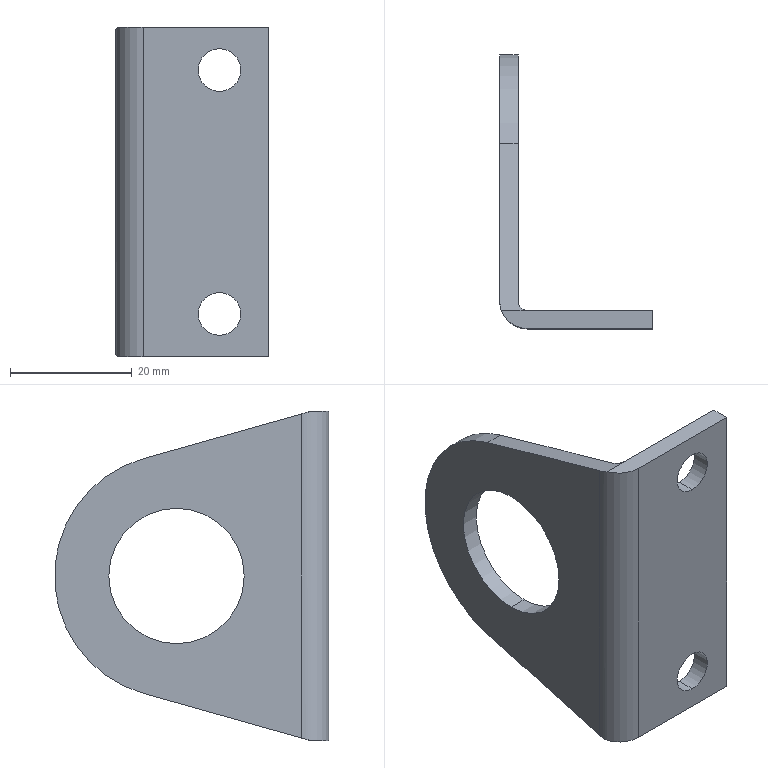Part | SolidWorks | features BaseBody 1 | 1 solid | 18 faces | box 25 x 45 x 54 mm | volume 7496 mm3 | cylinder 9 | plane 9 | commonest cylinder face diameters 7 x4 22.2 x2 3 x1 9 x1 40 x1
STEP:
#1=CARTESIAN_POINT('',(17.,-22.,16.5));
#2=VERTEX_POINT('',#1);
#3=CARTESIAN_POINT('',(17.,-22.,23.5));
#4=VERTEX_POINT('',#3);
#5=CARTESIAN_POINT('',(17.,-22.,20.));
#6=DIRECTION('',(0.,1.,0.));
#7=DIRECTION('',(1.,0.,0.));
#8=AXIS2_PLACEMENT_3D('',#5,#6,#7);
#9=CIRCLE('',#8,3.5);
#10=EDGE_CURVE('',#2,#4,#9,.T.);
#11=ORIENTED_EDGE('',*,*,#10,.T.);
#12=CARTESIAN_POINT('',(17.,-25.,23.5));
#13=VERTEX_POINT('',#12);
#14=CARTESIAN_POINT('',(17.,-22.,23.5));
#15=DIRECTION('',(0.,-1.,0.));
#16=VECTOR('',#15,1000.);
#17=LINE('',#14,#16);
#18=EDGE_CURVE('',#4,#13,#17,.T.);
#19=ORIENTED_EDGE('',*,*,#18,.T.);
#20=CARTESIAN_POINT('',(17.,-25.,16.5));
#21=VERTEX_POINT('',#20);
#22=CARTESIAN_POINT('',(17.,-25.,20.));
#23=DIRECTION('',(0.,-1.,0.));
#24=DIRECTION('',(0.,0.,1.));
#25=AXIS2_PLACEMENT_3D('',#22,#23,#24);
#26=CIRCLE('',#25,3.5);
#27=EDGE_CURVE('',#13,#21,#26,.T.);
#28=ORIENTED_EDGE('',*,*,#27,.T.);
#29=CARTESIAN_POINT('',(17.,-22.,16.5));
#30=DIRECTION('',(0.,-1.,0.));
#31=VECTOR('',#30,1000.);
#32=LINE('',#29,#31);
#33=EDGE_CURVE('',#2,#21,#32,.T.);
#34=ORIENTED_EDGE('',*,*,#33,.F.);
#35=EDGE_LOOP('',(#11,#19,#28,#34));
#36=FACE_OUTER_BOUND('',#35,.T.);
#37=CARTESIAN_POINT('',(17.,-22.,20.));
#38=DIRECTION('',(0.,-1.,0.));
#39=DIRECTION('',(0.,0.,-1.));
#40=AXIS2_PLACEMENT_3D('',#37,#38,#39);
#41=CYLINDRICAL_SURFACE('',#40,3.5);
#42=ADVANCED_FACE('',(#36),#41,.F.);
#43=CARTESIAN_POINT('',(17.,-22.,-23.5));
#44=VERTEX_POINT('',#43);
#45=CARTESIAN_POINT('',(17.,-22.,-16.5));
#46=VERTEX_POINT('',#45);
#47=CARTESIAN_POINT('',(17.,-22.,-20.));
#48=DIRECTION('',(0.,1.,0.));
#49=DIRECTION('',(1.,0.,0.));
#50=AXIS2_PLACEMENT_3D('',#47,#48,#49);
#51=CIRCLE('',#50,3.5);
#52=EDGE_CURVE('',#44,#46,#51,.T.);
#53=ORIENTED_EDGE('',*,*,#52,.T.);
#54=CARTESIAN_POINT('',(17.,-25.,-16.5));
#55=VERTEX_POINT('',#54);
#56=CARTESIAN_POINT('',(17.,-22.,-16.5));
#57=DIRECTION('',(0.,-1.,0.));
#58=VECTOR('',#57,1000.);
#59=LINE('',#56,#58);
#60=EDGE_CURVE('',#46,#55,#59,.T.);
#61=ORIENTED_EDGE('',*,*,#60,.T.);
#62=CARTESIAN_POINT('',(17.,-25.,-23.5));
#63=VERTEX_POINT('',#62);
#64=CARTESIAN_POINT('',(17.,-25.,-20.));
#65=DIRECTION('',(0.,-1.,0.));
#66=DIRECTION('',(0.,0.,1.));
#67=AXIS2_PLACEMENT_3D('',#64,#65,#66);
#68=CIRCLE('',#67,3.5);
#69=EDGE_CURVE('',#55,#63,#68,.T.);
#70=ORIENTED_EDGE('',*,*,#69,.T.);
#71=CARTESIAN_POINT('',(17.,-22.,-23.5));
#72=DIRECTION('',(0.,-1.,0.));
#73=VECTOR('',#72,1000.);
#74=LINE('',#71,#73);
#75=EDGE_CURVE('',#44,#63,#74,.T.);
#76=ORIENTED_EDGE('',*,*,#75,.F.);
#77=EDGE_LOOP('',(#53,#61,#70,#76));
#78=FACE_OUTER_BOUND('',#77,.T.);
#79=CARTESIAN_POINT('',(17.,-22.,-20.));
#80=DIRECTION('',(0.,-1.,0.));
#81=DIRECTION('',(0.,0.,-1.));
#82=AXIS2_PLACEMENT_3D('',#79,#80,#81);
#83=CYLINDRICAL_SURFACE('',#82,3.5);
#84=ADVANCED_FACE('',(#78),#83,.F.);
#85=CARTESIAN_POINT('',(3.,0.,11.1));
#86=VERTEX_POINT('',#85);
#87=CARTESIAN_POINT('',(3.,0.,-11.1));
#88=VERTEX_POINT('',#87);
#89=CARTESIAN_POINT('',(3.,0.,0.));
#90=DIRECTION('',(1.,0.,0.));
#91=DIRECTION('',(0.,0.,-1.));
#92=AXIS2_PLACEMENT_3D('',#89,#90,#91);
#93=CIRCLE('',#92,11.1);
#94=EDGE_CURVE('',#86,#88,#93,.T.);
#95=ORIENTED_EDGE('',*,*,#94,.T.);
#96=CARTESIAN_POINT('',(0.,0.,-11.1));
#97=VERTEX_POINT('',#96);
#98=CARTESIAN_POINT('',(3.,0.,-11.1));
#99=DIRECTION('',(-1.,0.,0.));
#100=VECTOR('',#99,1000.);
#101=LINE('',#98,#100);
#102=EDGE_CURVE('',#88,#97,#101,.T.);
#103=ORIENTED_EDGE('',*,*,#102,.T.);
#104=CARTESIAN_POINT('',(0.,0.,11.1));
#105=VERTEX_POINT('',#104);
#106=CARTESIAN_POINT('',(0.,0.,0.));
#107=DIRECTION('',(-1.,0.,0.));
#108=DIRECTION('',(0.,0.,-1.));
#109=AXIS2_PLACEMENT_3D('',#106,#107,#108);
#110=CIRCLE('',#109,11.1);
#111=EDGE_CURVE('',#97,#105,#110,.T.);
#112=ORIENTED_EDGE('',*,*,#111,.T.);
#113=CARTESIAN_POINT('',(3.,0.,11.1));
#114=DIRECTION('',(-1.,0.,0.));
#115=VECTOR('',#114,1000.);
#116=LINE('',#113,#115);
#117=EDGE_CURVE('',#86,#105,#116,.T.);
#118=ORIENTED_EDGE('',*,*,#117,.F.);
#119=EDGE_LOOP('',(#95,#103,#112,#118));
#120=FACE_OUTER_BOUND('',#119,.T.);
#121=CARTESIAN_POINT('',(3.,0.,0.));
#122=DIRECTION('',(-1.,0.,0.));
#123=DIRECTION('',(0.,0.,1.));
#124=AXIS2_PLACEMENT_3D('',#121,#122,#123);
#125=CYLINDRICAL_SURFACE('',#124,11.1);
#126=ADVANCED_FACE('',(#120),#125,.F.);
#127=CARTESIAN_POINT('',(0.,0.,0.));
#128=DIRECTION('',(-1.,0.,0.));
#129=DIRECTION('',(0.,0.,-1.));
#130=AXIS2_PLACEMENT_3D('',#127,#128,#129);
#131=CIRCLE('',#130,11.1);
#132=EDGE_CURVE('',#105,#97,#131,.T.);
#133=ORIENTED_EDGE('',*,*,#132,.F.);
#134=ORIENTED_EDGE('',*,*,#111,.F.);
#135=EDGE_LOOP('',(#133,#134));
#136=FACE_BOUND('',#135,.T.);
#137=CARTESIAN_POINT('',(0.,-20.5,26.576));
#138=VERTEX_POINT('',#137);
#139=CARTESIAN_POINT('',(0.,-20.5,-26.576));
#140=VERTEX_POINT('',#139);
#141=CARTESIAN_POINT('',(0.,-20.5,26.576));
#142=DIRECTION('',(0.,0.,-1.));
#143=VECTOR('',#142,1000.);
#144=LINE('',#141,#143);
#145=EDGE_CURVE('',#138,#140,#144,.T.);
#146=ORIENTED_EDGE('',*,*,#145,.F.);
#147=CARTESIAN_POINT('',(0.,5.439,19.246));
#148=VERTEX_POINT('',#147);
#149=CARTESIAN_POINT('',(0.,-20.5,26.576));
#150=DIRECTION('',(0.,0.9623,-0.2719));
#151=VECTOR('',#150,1000.);
#152=LINE('',#149,#151);
#153=EDGE_CURVE('',#138,#148,#152,.T.);
#154=ORIENTED_EDGE('',*,*,#153,.T.);
#155=CARTESIAN_POINT('',(0.,5.439,-19.246));
#156=VERTEX_POINT('',#155);
#157=CARTESIAN_POINT('',(0.,0.,0.));
#158=DIRECTION('',(-1.,0.,0.));
#159=DIRECTION('',(0.,0.2719,0.9623));
#160=AXIS2_PLACEMENT_3D('',#157,#158,#159);
#161=CIRCLE('',#160,20.);
#162=EDGE_CURVE('',#148,#156,#161,.T.);
#163=ORIENTED_EDGE('',*,*,#162,.T.);
#164=CARTESIAN_POINT('',(0.,5.439,-19.246));
#165=DIRECTION('',(0.,-0.9623,-0.2719));
#166=VECTOR('',#165,1000.);
#167=LINE('',#164,#166);
#168=EDGE_CURVE('',#156,#140,#167,.T.);
#169=ORIENTED_EDGE('',*,*,#168,.T.);
#170=EDGE_LOOP('',(#146,#154,#163,#169));
#171=FACE_OUTER_BOUND('',#170,.T.);
#172=CARTESIAN_POINT('',(0.,20.,27.));
#173=DIRECTION('',(1.,0.,0.));
#174=DIRECTION('',(0.,0.,-1.));
#175=AXIS2_PLACEMENT_3D('',#172,#173,#174);
#176=PLANE('',#175);
#177=ADVANCED_FACE('',(#136,#171),#176,.F.);
#178=CARTESIAN_POINT('',(0.2574,-22.,27.));
#179=VERTEX_POINT('',#178);
#180=CARTESIAN_POINT('',(4.5,-25.,27.));
#181=VERTEX_POINT('',#180);
#182=CARTESIAN_POINT('',(4.5,-20.5,27.));
#183=DIRECTION('',(0.,0.,1.));
#184=DIRECTION('',(-0.9428,-0.3333,0.));
#185=AXIS2_PLACEMENT_3D('',#182,#183,#184);
#186=CIRCLE('',#185,4.5);
#187=EDGE_CURVE('',#179,#181,#186,.T.);
#188=ORIENTED_EDGE('',*,*,#187,.F.);
#189=CARTESIAN_POINT('',(0.2574,-22.,27.));
#190=CARTESIAN_POINT('',(0.08715,-21.519,26.864));
#191=CARTESIAN_POINT('',(0.,-21.01,26.72));
#192=CARTESIAN_POINT('',(0.,-20.5,26.576));
#193=B_SPLINE_CURVE_WITH_KNOTS('',3,(#189,#190,#191,#192),.UNSPECIFIED.,.F.,.F.,(4,4),(4.373,4.712),.UNSPECIFIED.);
#194=EDGE_CURVE('',#179,#138,#193,.T.);
#195=ORIENTED_EDGE('',*,*,#194,.T.);
#196=ORIENTED_EDGE('',*,*,#145,.T.);
#197=CARTESIAN_POINT('',(0.2574,-22.,-27.));
#198=VERTEX_POINT('',#197);
#199=CARTESIAN_POINT('',(0.,-20.5,-26.576));
#200=CARTESIAN_POINT('',(0.,-21.01,-26.72));
#201=CARTESIAN_POINT('',(0.08715,-21.519,-26.864));
#202=CARTESIAN_POINT('',(0.2574,-22.,-27.));
#203=B_SPLINE_CURVE_WITH_KNOTS('',3,(#199,#200,#201,#202),.UNSPECIFIED.,.F.,.F.,(4,4),(4.712,5.052),.UNSPECIFIED.);
#204=EDGE_CURVE('',#140,#198,#203,.T.);
#205=ORIENTED_EDGE('',*,*,#204,.T.);
#206=CARTESIAN_POINT('',(4.5,-25.,-27.));
#207=VERTEX_POINT('',#206);
#208=CARTESIAN_POINT('',(4.5,-20.5,-27.));
#209=DIRECTION('',(0.,0.,1.));
#210=DIRECTION('',(-0.9428,-0.3333,0.));
#211=AXIS2_PLACEMENT_3D('',#208,#209,#210);
#212=CIRCLE('',#211,4.5);
#213=EDGE_CURVE('',#198,#207,#212,.T.);
#214=ORIENTED_EDGE('',*,*,#213,.T.);
#215=CARTESIAN_POINT('',(4.5,-25.,27.));
#216=DIRECTION('',(0.,0.,-1.));
#217=VECTOR('',#216,1000.);
#218=LINE('',#215,#217);
#219=EDGE_CURVE('',#181,#207,#218,.T.);
#220=ORIENTED_EDGE('',*,*,#219,.F.);
#221=EDGE_LOOP('',(#188,#195,#196,#205,#214,#220));
#222=FACE_OUTER_BOUND('',#221,.T.);
#223=CARTESIAN_POINT('',(4.5,-20.5,27.));
#224=DIRECTION('',(0.,0.,-1.));
#225=DIRECTION('',(-1.,0.,0.));
#226=AXIS2_PLACEMENT_3D('',#223,#224,#225);
#227=CYLINDRICAL_SURFACE('',#226,4.5);
#228=ADVANCED_FACE('',(#222),#227,.T.);
#229=CARTESIAN_POINT('',(17.,-25.,20.));
#230=DIRECTION('',(0.,-1.,0.));
#231=DIRECTION('',(0.,0.,1.));
#232=AXIS2_PLACEMENT_3D('',#229,#230,#231);
#233=CIRCLE('',#232,3.5);
#234=EDGE_CURVE('',#21,#13,#233,.T.);
#235=ORIENTED_EDGE('',*,*,#234,.F.);
#236=ORIENTED_EDGE('',*,*,#27,.F.);
#237=EDGE_LOOP('',(#235,#236));
#238=FACE_BOUND('',#237,.T.);
#239=CARTESIAN_POINT('',(17.,-25.,-20.));
#240=DIRECTION('',(0.,-1.,0.));
#241=DIRECTION('',(0.,0.,1.));
#242=AXIS2_PLACEMENT_3D('',#239,#240,#241);
#243=CIRCLE('',#242,3.5);
#244=EDGE_CURVE('',#63,#55,#243,.T.);
#245=ORIENTED_EDGE('',*,*,#244,.F.);
#246=ORIENTED_EDGE('',*,*,#69,.F.);
#247=EDGE_LOOP('',(#245,#246));
#248=FACE_BOUND('',#247,.T.);
#249=CARTESIAN_POINT('',(25.,-25.,27.));
#250=VERTEX_POINT('',#249);
#251=CARTESIAN_POINT('',(25.,-25.,-27.));
#252=VERTEX_POINT('',#251);
#253=CARTESIAN_POINT('',(25.,-25.,27.));
#254=DIRECTION('',(0.,0.,-1.));
#255=VECTOR('',#254,1000.);
#256=LINE('',#253,#255);
#257=EDGE_CURVE('',#250,#252,#256,.T.);
#258=ORIENTED_EDGE('',*,*,#257,.F.);
#259=CARTESIAN_POINT('',(4.5,-25.,27.));
#260=DIRECTION('',(1.,0.,0.));
#261=VECTOR('',#260,1000.);
#262=LINE('',#259,#261);
#263=EDGE_CURVE('',#181,#250,#262,.T.);
#264=ORIENTED_EDGE('',*,*,#263,.F.);
#265=ORIENTED_EDGE('',*,*,#219,.T.);
#266=CARTESIAN_POINT('',(4.5,-25.,-27.));
#267=DIRECTION('',(1.,0.,0.));
#268=VECTOR('',#267,1000.);
#269=LINE('',#266,#268);
#270=EDGE_CURVE('',#207,#252,#269,.T.);
#271=ORIENTED_EDGE('',*,*,#270,.T.);
#272=EDGE_LOOP('',(#258,#264,#265,#271));
#273=FACE_OUTER_BOUND('',#272,.T.);
#274=CARTESIAN_POINT('',(4.5,-25.,27.));
#275=DIRECTION('',(0.,1.,0.));
#276=DIRECTION('',(0.,0.,1.));
#277=AXIS2_PLACEMENT_3D('',#274,#275,#276);
#278=PLANE('',#277);
#279=ADVANCED_FACE('',(#238,#248,#273),#278,.F.);
#280=CARTESIAN_POINT('',(25.,-22.,-27.));
#281=VERTEX_POINT('',#280);
#282=CARTESIAN_POINT('',(25.,-25.,-27.));
#283=DIRECTION('',(0.,1.,0.));
#284=VECTOR('',#283,1000.);
#285=LINE('',#282,#284);
#286=EDGE_CURVE('',#252,#281,#285,.T.);
#287=ORIENTED_EDGE('',*,*,#286,.T.);
#288=CARTESIAN_POINT('',(25.,-22.,27.));
#289=VERTEX_POINT('',#288);
#290=CARTESIAN_POINT('',(25.,-22.,27.));
#291=DIRECTION('',(0.,0.,-1.));
#292=VECTOR('',#291,1000.);
#293=LINE('',#290,#292);
#294=EDGE_CURVE('',#289,#281,#293,.T.);
#295=ORIENTED_EDGE('',*,*,#294,.F.);
#296=CARTESIAN_POINT('',(25.,-25.,27.));
#297=DIRECTION('',(0.,1.,0.));
#298=VECTOR('',#297,1000.);
#299=LINE('',#296,#298);
#300=EDGE_CURVE('',#250,#289,#299,.T.);
#301=ORIENTED_EDGE('',*,*,#300,.F.);
#302=ORIENTED_EDGE('',*,*,#257,.T.);
#303=EDGE_LOOP('',(#287,#295,#301,#302));
#304=FACE_OUTER_BOUND('',#303,.T.);
#305=CARTESIAN_POINT('',(25.,-25.,27.));
#306=DIRECTION('',(-1.,0.,0.));
#307=DIRECTION('',(0.,0.,1.));
#308=AXIS2_PLACEMENT_3D('',#305,#306,#307);
#309=PLANE('',#308);
#310=ADVANCED_FACE('',(#304),#309,.F.);
#311=ORIENTED_EDGE('',*,*,#10,.F.);
#312=CARTESIAN_POINT('',(17.,-22.,20.));
#313=DIRECTION('',(0.,1.,0.));
#314=DIRECTION('',(1.,0.,0.));
#315=AXIS2_PLACEMENT_3D('',#312,#313,#314);
#316=CIRCLE('',#315,3.5);
#317=EDGE_CURVE('',#4,#2,#316,.T.);
#318=ORIENTED_EDGE('',*,*,#317,.F.);
#319=EDGE_LOOP('',(#311,#318));
#320=FACE_BOUND('',#319,.T.);
#321=ORIENTED_EDGE('',*,*,#52,.F.);
#322=CARTESIAN_POINT('',(17.,-22.,-20.));
#323=DIRECTION('',(0.,1.,0.));
#324=DIRECTION('',(1.,0.,0.));
#325=AXIS2_PLACEMENT_3D('',#322,#323,#324);
#326=CIRCLE('',#325,3.5);
#327=EDGE_CURVE('',#46,#44,#326,.T.);
#328=ORIENTED_EDGE('',*,*,#327,.F.);
#329=EDGE_LOOP('',(#321,#328));
#330=FACE_BOUND('',#329,.T.);
#331=CARTESIAN_POINT('',(4.5,-22.,-27.));
#332=VERTEX_POINT('',#331);
#333=CARTESIAN_POINT('',(25.,-22.,-27.));
#334=DIRECTION('',(-1.,0.,0.));
#335=VECTOR('',#334,1000.);
#336=LINE('',#333,#335);
#337=EDGE_CURVE('',#281,#332,#336,.T.);
#338=ORIENTED_EDGE('',*,*,#337,.T.);
#339=CARTESIAN_POINT('',(4.5,-22.,27.));
#340=VERTEX_POINT('',#339);
#341=CARTESIAN_POINT('',(4.5,-22.,27.));
#342=DIRECTION('',(0.,0.,-1.));
#343=VECTOR('',#342,1000.);
#344=LINE('',#341,#343);
#345=EDGE_CURVE('',#340,#332,#344,.T.);
#346=ORIENTED_EDGE('',*,*,#345,.F.);
#347=CARTESIAN_POINT('',(25.,-22.,27.));
#348=DIRECTION('',(-1.,0.,0.));
#349=VECTOR('',#348,1000.);
#350=LINE('',#347,#349);
#351=EDGE_CURVE('',#289,#340,#350,.T.);
#352=ORIENTED_EDGE('',*,*,#351,.F.);
#353=ORIENTED_EDGE('',*,*,#294,.T.);
#354=EDGE_LOOP('',(#338,#346,#352,#353));
#355=FACE_OUTER_BOUND('',#354,.T.);
#356=CARTESIAN_POINT('',(25.,-22.,27.));
#357=DIRECTION('',(0.,-1.,0.));
#358=DIRECTION('',(0.,0.,-1.));
#359=AXIS2_PLACEMENT_3D('',#356,#357,#358);
#360=PLANE('',#359);
#361=ADVANCED_FACE('',(#320,#330,#355),#360,.F.);
#362=CARTESIAN_POINT('',(3.,-20.5,26.576));
#363=VERTEX_POINT('',#362);
#364=CARTESIAN_POINT('',(4.5,-22.,27.));
#365=CARTESIAN_POINT('',(4.3,-22.,27.));
#366=CARTESIAN_POINT('',(4.11,-21.962,26.989));
#367=CARTESIAN_POINT('',(3.742,-21.81,26.946));
#368=CARTESIAN_POINT('',(3.58,-21.701,26.916));
#369=CARTESIAN_POINT('',(3.299,-21.42,26.836));
#370=CARTESIAN_POINT('',(3.19,-21.257,26.79));
#371=CARTESIAN_POINT('',(3.038,-20.891,26.687));
#372=CARTESIAN_POINT('',(3.,-20.698,26.632));
#373=CARTESIAN_POINT('',(3.,-20.5,26.576));
#374=B_SPLINE_CURVE_WITH_KNOTS('',3,(#364,#365,#366,#367,#368,#369,#370,#371,#372,#373),.UNSPECIFIED.,.F.,.F.,(4,2,2,2,4),(3.142,3.534,3.927,4.32,4.712),.UNSPECIFIED.);
#375=EDGE_CURVE('',#340,#363,#374,.T.);
#376=ORIENTED_EDGE('',*,*,#375,.F.);
#377=ORIENTED_EDGE('',*,*,#345,.T.);
#378=CARTESIAN_POINT('',(3.,-20.5,-26.576));
#379=VERTEX_POINT('',#378);
#380=CARTESIAN_POINT('',(3.,-20.5,-26.576));
#381=CARTESIAN_POINT('',(3.,-20.698,-26.632));
#382=CARTESIAN_POINT('',(3.038,-20.891,-26.687));
#383=CARTESIAN_POINT('',(3.19,-21.257,-26.79));
#384=CARTESIAN_POINT('',(3.299,-21.42,-26.836));
#385=CARTESIAN_POINT('',(3.58,-21.701,-26.916));
#386=CARTESIAN_POINT('',(3.742,-21.81,-26.946));
#387=CARTESIAN_POINT('',(4.11,-21.962,-26.989));
#388=CARTESIAN_POINT('',(4.3,-22.,-27.));
#389=CARTESIAN_POINT('',(4.5,-22.,-27.));
#390=B_SPLINE_CURVE_WITH_KNOTS('',3,(#380,#381,#382,#383,#384,#385,#386,#387,#388,#389),.UNSPECIFIED.,.F.,.F.,(4,2,2,2,4),(4.712,5.105,5.498,5.89,6.283),.UNSPECIFIED.);
#391=EDGE_CURVE('',#379,#332,#390,.T.);
#392=ORIENTED_EDGE('',*,*,#391,.F.);
#393=CARTESIAN_POINT('',(3.,-20.5,26.576));
#394=DIRECTION('',(0.,0.,-1.));
#395=VECTOR('',#394,1000.);
#396=LINE('',#393,#395);
#397=EDGE_CURVE('',#363,#379,#396,.T.);
#398=ORIENTED_EDGE('',*,*,#397,.F.);
#399=EDGE_LOOP('',(#376,#377,#392,#398));
#400=FACE_OUTER_BOUND('',#399,.T.);
#401=CARTESIAN_POINT('',(4.5,-20.5,27.));
#402=DIRECTION('',(0.,0.,-1.));
#403=DIRECTION('',(-1.,0.,0.));
#404=AXIS2_PLACEMENT_3D('',#401,#402,#403);
#405=CYLINDRICAL_SURFACE('',#404,1.5);
#406=ADVANCED_FACE('',(#400),#405,.F.);
#407=ORIENTED_EDGE('',*,*,#94,.F.);
#408=CARTESIAN_POINT('',(3.,0.,0.));
#409=DIRECTION('',(1.,0.,0.));
#410=DIRECTION('',(0.,0.,-1.));
#411=AXIS2_PLACEMENT_3D('',#408,#409,#410);
#412=CIRCLE('',#411,11.1);
#413=EDGE_CURVE('',#88,#86,#412,.T.);
#414=ORIENTED_EDGE('',*,*,#413,.F.);
#415=EDGE_LOOP('',(#407,#414));
#416=FACE_BOUND('',#415,.T.);
#417=CARTESIAN_POINT('',(3.,5.439,-19.246));
#418=VERTEX_POINT('',#417);
#419=CARTESIAN_POINT('',(3.,5.439,19.246));
#420=VERTEX_POINT('',#419);
#421=CARTESIAN_POINT('',(3.,0.,0.));
#422=DIRECTION('',(1.,0.,0.));
#423=DIRECTION('',(0.,0.2719,-0.9623));
#424=AXIS2_PLACEMENT_3D('',#421,#422,#423);
#425=CIRCLE('',#424,20.);
#426=EDGE_CURVE('',#418,#420,#425,.T.);
#427=ORIENTED_EDGE('',*,*,#426,.T.);
#428=CARTESIAN_POINT('',(3.,5.439,19.246));
#429=DIRECTION('',(0.,-0.9623,0.2719));
#430=VECTOR('',#429,1000.);
#431=LINE('',#428,#430);
#432=EDGE_CURVE('',#420,#363,#431,.T.);
#433=ORIENTED_EDGE('',*,*,#432,.T.);
#434=ORIENTED_EDGE('',*,*,#397,.T.);
#435=CARTESIAN_POINT('',(3.,-20.5,-26.576));
#436=DIRECTION('',(0.,0.9623,0.2719));
#437=VECTOR('',#436,1000.);
#438=LINE('',#435,#437);
#439=EDGE_CURVE('',#379,#418,#438,.T.);
#440=ORIENTED_EDGE('',*,*,#439,.T.);
#441=EDGE_LOOP('',(#427,#433,#434,#440));
#442=FACE_OUTER_BOUND('',#441,.T.);
#443=CARTESIAN_POINT('',(3.,-20.5,27.));
#444=DIRECTION('',(-1.,0.,0.));
#445=DIRECTION('',(0.,0.,1.));
#446=AXIS2_PLACEMENT_3D('',#443,#444,#445);
#447=PLANE('',#446);
#448=ADVANCED_FACE('',(#416,#442),#447,.F.);
#449=ORIENTED_EDGE('',*,*,#351,.T.);
#450=CARTESIAN_POINT('',(4.5,-22.,27.));
#451=DIRECTION('',(-1.,0.,0.));
#452=VECTOR('',#451,1000.);
#453=LINE('',#450,#452);
#454=EDGE_CURVE('',#340,#179,#453,.T.);
#455=ORIENTED_EDGE('',*,*,#454,.T.);
#456=ORIENTED_EDGE('',*,*,#187,.T.);
#457=ORIENTED_EDGE('',*,*,#263,.T.);
#458=ORIENTED_EDGE('',*,*,#300,.T.);
#459=EDGE_LOOP('',(#449,#455,#456,#457,#458));
#460=FACE_OUTER_BOUND('',#459,.T.);
#461=CARTESIAN_POINT('',(4.5,-20.5,27.));
#462=DIRECTION('',(0.,0.,1.));
#463=DIRECTION('',(1.,0.,0.));
#464=AXIS2_PLACEMENT_3D('',#461,#462,#463);
#465=PLANE('',#464);
#466=ADVANCED_FACE('',(#460),#465,.T.);
#467=ORIENTED_EDGE('',*,*,#286,.F.);
#468=ORIENTED_EDGE('',*,*,#270,.F.);
#469=ORIENTED_EDGE('',*,*,#213,.F.);
#470=CARTESIAN_POINT('',(4.5,-22.,-27.));
#471=DIRECTION('',(-1.,0.,0.));
#472=VECTOR('',#471,1000.);
#473=LINE('',#470,#472);
#474=EDGE_CURVE('',#332,#198,#473,.T.);
#475=ORIENTED_EDGE('',*,*,#474,.F.);
#476=ORIENTED_EDGE('',*,*,#337,.F.);
#477=EDGE_LOOP('',(#467,#468,#469,#475,#476));
#478=FACE_OUTER_BOUND('',#477,.T.);
#479=CARTESIAN_POINT('',(4.5,-20.5,-27.));
#480=DIRECTION('',(0.,0.,1.));
#481=DIRECTION('',(1.,0.,0.));
#482=AXIS2_PLACEMENT_3D('',#479,#480,#481);
#483=PLANE('',#482);
#484=ADVANCED_FACE('',(#478),#483,.F.);
#485=ORIENTED_EDGE('',*,*,#102,.F.);
#486=ORIENTED_EDGE('',*,*,#413,.T.);
#487=ORIENTED_EDGE('',*,*,#117,.T.);
#488=ORIENTED_EDGE('',*,*,#132,.T.);
#489=EDGE_LOOP('',(#485,#486,#487,#488));
#490=FACE_OUTER_BOUND('',#489,.T.);
#491=CARTESIAN_POINT('',(3.,0.,0.));
#492=DIRECTION('',(-1.,0.,0.));
#493=DIRECTION('',(0.,0.,1.));
#494=AXIS2_PLACEMENT_3D('',#491,#492,#493);
#495=CYLINDRICAL_SURFACE('',#494,11.1);
#496=ADVANCED_FACE('',(#490),#495,.F.);
#497=CARTESIAN_POINT('',(3.,5.439,19.246));
#498=DIRECTION('',(-1.,0.,0.));
#499=VECTOR('',#498,1000.);
#500=LINE('',#497,#499);
#501=EDGE_CURVE('',#420,#148,#500,.T.);
#502=ORIENTED_EDGE('',*,*,#501,.F.);
#503=ORIENTED_EDGE('',*,*,#426,.F.);
#504=CARTESIAN_POINT('',(3.,5.439,-19.246));
#505=DIRECTION('',(-1.,0.,0.));
#506=VECTOR('',#505,1000.);
#507=LINE('',#504,#506);
#508=EDGE_CURVE('',#418,#156,#507,.T.);
#509=ORIENTED_EDGE('',*,*,#508,.T.);
#510=ORIENTED_EDGE('',*,*,#162,.F.);
#511=EDGE_LOOP('',(#502,#503,#509,#510));
#512=FACE_OUTER_BOUND('',#511,.T.);
#513=CARTESIAN_POINT('',(17.,0.,0.));
#514=DIRECTION('',(-1.,0.,0.));
#515=DIRECTION('',(0.,0.,1.));
#516=AXIS2_PLACEMENT_3D('',#513,#514,#515);
#517=CYLINDRICAL_SURFACE('',#516,20.);
#518=ADVANCED_FACE('',(#512),#517,.T.);
#519=ORIENTED_EDGE('',*,*,#194,.F.);
#520=ORIENTED_EDGE('',*,*,#454,.F.);
#521=ORIENTED_EDGE('',*,*,#375,.T.);
#522=ORIENTED_EDGE('',*,*,#432,.F.);
#523=ORIENTED_EDGE('',*,*,#501,.T.);
#524=ORIENTED_EDGE('',*,*,#153,.F.);
#525=EDGE_LOOP('',(#519,#520,#521,#522,#523,#524));
#526=FACE_OUTER_BOUND('',#525,.T.);
#527=CARTESIAN_POINT('',(17.,5.439,19.246));
#528=DIRECTION('',(0.,-0.2719,-0.9623));
#529=DIRECTION('',(0.,0.9623,-0.2719));
#530=AXIS2_PLACEMENT_3D('',#527,#528,#529);
#531=PLANE('',#530);
#532=ADVANCED_FACE('',(#526),#531,.F.);
#533=ORIENTED_EDGE('',*,*,#508,.F.);
#534=ORIENTED_EDGE('',*,*,#439,.F.);
#535=ORIENTED_EDGE('',*,*,#391,.T.);
#536=ORIENTED_EDGE('',*,*,#474,.T.);
#537=ORIENTED_EDGE('',*,*,#204,.F.);
#538=ORIENTED_EDGE('',*,*,#168,.F.);
#539=EDGE_LOOP('',(#533,#534,#535,#536,#537,#538));
#540=FACE_OUTER_BOUND('',#539,.T.);
#541=CARTESIAN_POINT('',(17.,-22.,-27.));
#542=DIRECTION('',(0.,-0.2719,0.9623));
#543=DIRECTION('',(0.,-0.9623,-0.2719));
#544=AXIS2_PLACEMENT_3D('',#541,#542,#543);
#545=PLANE('',#544);
#546=ADVANCED_FACE('',(#540),#545,.F.);
#547=ORIENTED_EDGE('',*,*,#60,.F.);
#548=ORIENTED_EDGE('',*,*,#327,.T.);
#549=ORIENTED_EDGE('',*,*,#75,.T.);
#550=ORIENTED_EDGE('',*,*,#244,.T.);
#551=EDGE_LOOP('',(#547,#548,#549,#550));
#552=FACE_OUTER_BOUND('',#551,.T.);
#553=CARTESIAN_POINT('',(17.,-22.,-20.));
#554=DIRECTION('',(0.,-1.,0.));
#555=DIRECTION('',(0.,0.,-1.));
#556=AXIS2_PLACEMENT_3D('',#553,#554,#555);
#557=CYLINDRICAL_SURFACE('',#556,3.5);
#558=ADVANCED_FACE('',(#552),#557,.F.);
#559=ORIENTED_EDGE('',*,*,#18,.F.);
#560=ORIENTED_EDGE('',*,*,#317,.T.);
#561=ORIENTED_EDGE('',*,*,#33,.T.);
#562=ORIENTED_EDGE('',*,*,#234,.T.);
#563=EDGE_LOOP('',(#559,#560,#561,#562));
#564=FACE_OUTER_BOUND('',#563,.T.);
#565=CARTESIAN_POINT('',(17.,-22.,20.));
#566=DIRECTION('',(0.,-1.,0.));
#567=DIRECTION('',(0.,0.,-1.));
#568=AXIS2_PLACEMENT_3D('',#565,#566,#567);
#569=CYLINDRICAL_SURFACE('',#568,3.5);
#570=ADVANCED_FACE('',(#564),#569,.F.);
#571=CLOSED_SHELL('',(#42,#84,#126,#177,#228,#279,#310,#361,#406,#448,#466,#484,#496,#518,#532,#546,#558,#570));
#572=MANIFOLD_SOLID_BREP('',#571);
#573=CARTESIAN_POINT('',(0.,0.,0.));
#574=DIRECTION('',(0.,0.,1.));
#575=DIRECTION('',(1.,0.,0.));
#576=AXIS2_PLACEMENT_3D('',#573,#574,#575);
#577=(LENGTH_UNIT()NAMED_UNIT(*)SI_UNIT(.MILLI.,.METRE.));
#578=UNCERTAINTY_MEASURE_WITH_UNIT(LENGTH_MEASURE(0.00001),#577,'','');
#579=(NAMED_UNIT(*)PLANE_ANGLE_UNIT()SI_UNIT($,.RADIAN.));
#580=(NAMED_UNIT(*)SI_UNIT($,.STERADIAN.)SOLID_ANGLE_UNIT());
#581=(GEOMETRIC_REPRESENTATION_CONTEXT(3)GLOBAL_UNCERTAINTY_ASSIGNED_CONTEXT((#578))GLOBAL_UNIT_ASSIGNED_CONTEXT((#577,#579,#580))REPRESENTATION_CONTEXT('',''));
#582=ADVANCED_BREP_SHAPE_REPRESENTATION('',(#572,#576),#581);